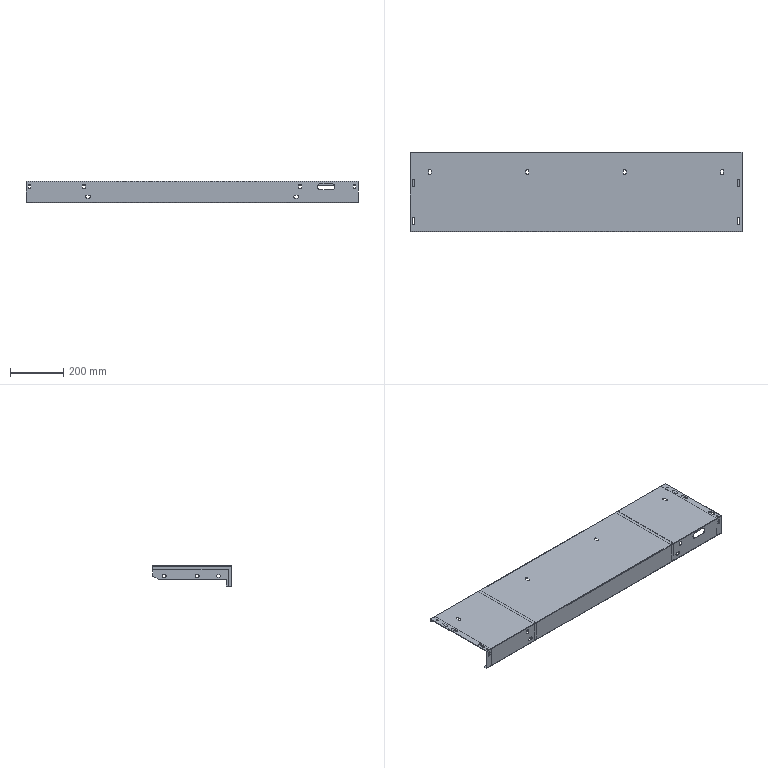Part | SolidWorks | features MirrorCompFeat 2, ReferencePattern 2 | 5 solids | 291 faces | box 1250 x 299.5 x 80 mm | volume 853171 mm3 | plane 196 | cylinder 95 | commonest cylinder face diameters 10 x32 9 x20 6 x12 11 x10 0.4 x7 2 x4